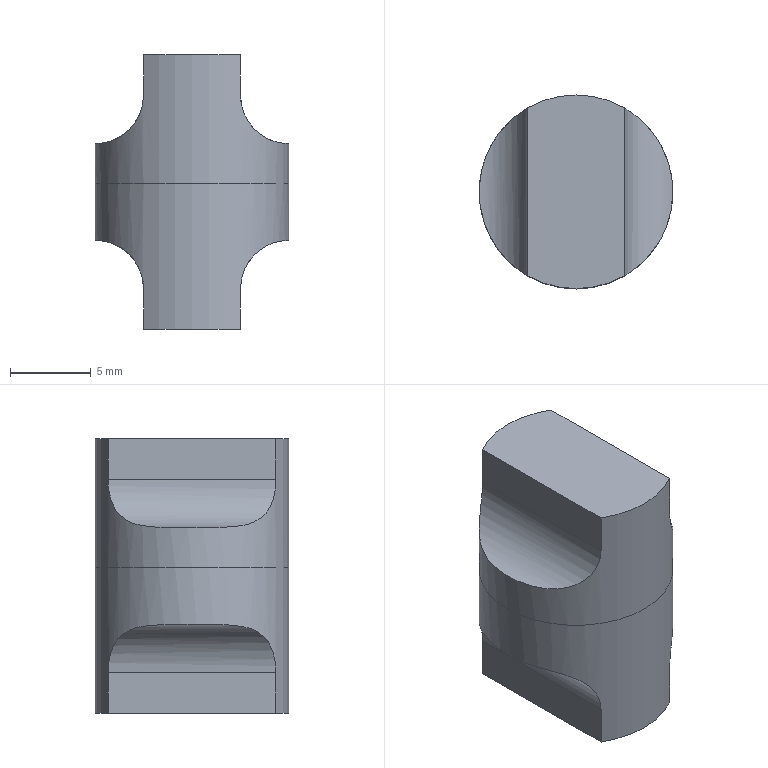CAM job | NX | 3-axis milling, drilling | part box 12 x 12 x 17 mm | stock box 15 x 15 x 23 mm
Tools:
number,name,description,diameter,corner_radius,flute_length,length,flutes
1,D8开粗,,8.0,0.0,50.0,75.0,2
5,D6倒角刀,,6.0,0.0,50.0,75.0,2
7,D8R3,,8.0,3.0,50.0,75.0,2
2,D8精光,,8.0,0.0,50.0,75.0,2
3,D10点钻,,10.0,0.0,50.0,75.0,2
4,5.1钻头,,5.1,0.0,50.0,75.0,2
6,6-1,,4.3,0.0,1.0,50.0,2
Operations:
program,operation,operation_type,tool,method,geometry_group,spindle_rpm,surface_speed,feed_per_tooth,feed_cut,feed_plunge,cut_length_mm,path_length_mm,cut_time_min,machine_time_min
G54,PLANAR_MILL,PlanarMilling,D8开粗,METHOD,WORKPIECE,2000.0,50.0,0.2,800.0,100.0,28.392,64.292,0.0355,0.0391
G54,ADAPTIVE_MILLING,CavityMilling,D8开粗,METHOD,WORKPIECE,3000.0,75.0,0.1667,1000.0,100.0,1102.48,1517.716,0.8882,0.9297
G54,PLANAR_MILL_3,PlanarMilling,D6倒角刀,METHOD,WORKPIECE,3000.0,56.0,0.1333,800.0,100.0,44.785,134.185,0.056,0.0649
G54,PLANAR_MILL_3_COPY,PlanarMilling,D6倒角刀,METHOD,WORKPIECE,3000.0,56.0,0.1333,800.0,100.0,40.755,130.612,0.0509,0.0599
G54,PLANAR_MILL_2,PlanarMilling,D8R3,METHOD,WORKPIECE,3000.0,75.0,0.1,600.0,100.0,105.569,250.354,0.1759,0.1904
G54,PLANAR_MILL_COPY,PlanarMilling,D8精光,METHOD,WORKPIECE,3000.0,75.0,0.1,600.0,100.0,28.392,64.392,0.0473,0.0509
G54,PLANAR_MILL_1,PlanarMilling,D8精光,METHOD,WORKPIECE,3000.0,75.0,0.1,600.0,100.0,146.23,205.23,0.2437,0.2496
G55,ADAPTIVE_MILLING_1,CavityMilling,D8开粗,METHOD,WORKPIECE_1,2500.0,62.0,0.2,1000.0,100.0,949.022,1022.28,0.949,0.9563
G55,PLANAR_MILL_6,PlanarMilling,D6倒角刀,METHOD,WORKPIECE_1,3000.0,56.0,0.1,600.0,100.0,44.841,83.841,0.0747,0.0786
G55,PLANAR_MILL_6_COPY,PlanarMilling,D6倒角刀,METHOD,WORKPIECE_1,3000.0,56.0,0.1,600.0,100.0,57.407,101.407,0.0957,0.1001
G55,DRILLING,Operation,D10点钻,METHOD,WORKPIECE_1,1200.0,37.0,0.0417,100.0,0.0,4.5,49.0,0.045,0.0494
G55,DRILLING_1,Operation,5.1钻头,METHOD,WORKPIECE_1,1600.0,25.0,0.0469,150.0,0.0,10.5,61.0,0.07,0.075
G55,DRILLING_COPY,Operation,D10点钻,METHOD,WORKPIECE_1,1600.0,25.0,0.0469,150.0,0.0,6.0,52.0,0.04,0.0446
G55,PLANAR_MILL_4,PlanarMilling,D8精光,METHOD,WORKPIECE_1,3000.0,56.0,0.1,600.0,100.0,32.392,66.392,0.054,0.0574
G55,PLANAR_MILL_5,PlanarMilling,D8精光,METHOD,WORKPIECE_1,3000.0,56.0,0.1,600.0,100.0,120.276,161.276,0.2005,0.2046
G55,THREAD_MILLING,ThreadMilling,6-1,METHOD,WORKPIECE_1,3500.0,43.0,0.0143,100.0,100.0,80.31,258.31,0.8031,0.8209
G56,PLANAR_MILL_COPY_1_COPY_COPY,PlanarMilling,D8开粗,METHOD,WORKPIECE_2,2000.0,50.0,0.2,800.0,100.0,28.392,64.292,0.0355,0.0391
G56,ADAPTIVE_MILLING_1_COPY,CavityMilling,D8开粗,METHOD,WORKPIECE_2,2500.0,62.0,0.2,1000.0,100.0,1210.768,1969.834,1.021,1.097
G56,PLANAR_MILL_COPY_1_COPY,PlanarMilling,D8精光,METHOD,WORKPIECE_2,2000.0,50.0,0.2,800.0,100.0,28.392,64.392,0.0355,0.0391
G56,PLANAR_MILL_2_COPY,PlanarMilling,D8R3,METHOD,WORKPIECE_2,3000.0,75.0,0.1,600.0,100.0,105.569,250.354,0.1759,0.1904
G56,PLANAR_MILL_3_COPY_1,PlanarMilling,D6倒角刀,METHOD,WORKPIECE_2,3000.0,56.0,0.1333,800.0,100.0,44.785,134.185,0.056,0.0649
G56,PLANAR_MILL_3_COPY_COPY_1,PlanarMilling,D6倒角刀,METHOD,WORKPIECE_2,3000.0,56.0,0.1333,800.0,100.0,40.755,130.612,0.0509,0.0599
G56,PLANAR_MILL_1_COPY_COPY,PlanarMilling,D8精光,METHOD,WORKPIECE_2,3000.0,75.0,0.1,600.0,100.0,146.23,202.23,0.2437,0.2493
G57,ADAPTIVE_MILLING_COPY,CavityMilling,D8开粗,METHOD,WORKPIECE_3,3000.0,75.0,0.1667,1000.0,100.0,895.927,929.927,0.8959,0.8993
G57,DRILLING_COPY_1,Operation,D10点钻,METHOD,WORKPIECE_3,1200.0,37.0,0.0417,100.0,0.0,4.0,48.0,0.04,0.0444
G57,DRILLING_1_COPY,Operation,5.1钻头,METHOD,WORKPIECE_3,1600.0,25.0,0.0469,150.0,0.0,9.0,58.0,0.06,0.0649
G57,DRILLING_COPY_1_COPY,Operation,D10点钻,METHOD,WORKPIECE_3,1200.0,37.0,0.0417,100.0,0.0,6.0,52.0,0.06,0.0646
G57,THREAD_MILLING_COPY,ThreadMilling,6-1,METHOD,WORKPIECE_3,3500.0,43.0,0.0143,100.0,100.0,74.546,250.547,0.7455,0.7631
G57,PLANAR_MILL_3_COPY_COPY,PlanarMilling,D6倒角刀,METHOD,WORKPIECE_3,3000.0,56.0,0.1333,800.0,100.0,60.549,100.549,0.0757,0.0797
G57,PLANAR_MILL_COPY_COPY,PlanarMilling,D8精光,METHOD,WORKPIECE_3,3000.0,75.0,0.1,600.0,100.0,56.785,153.811,0.0946,0.1043